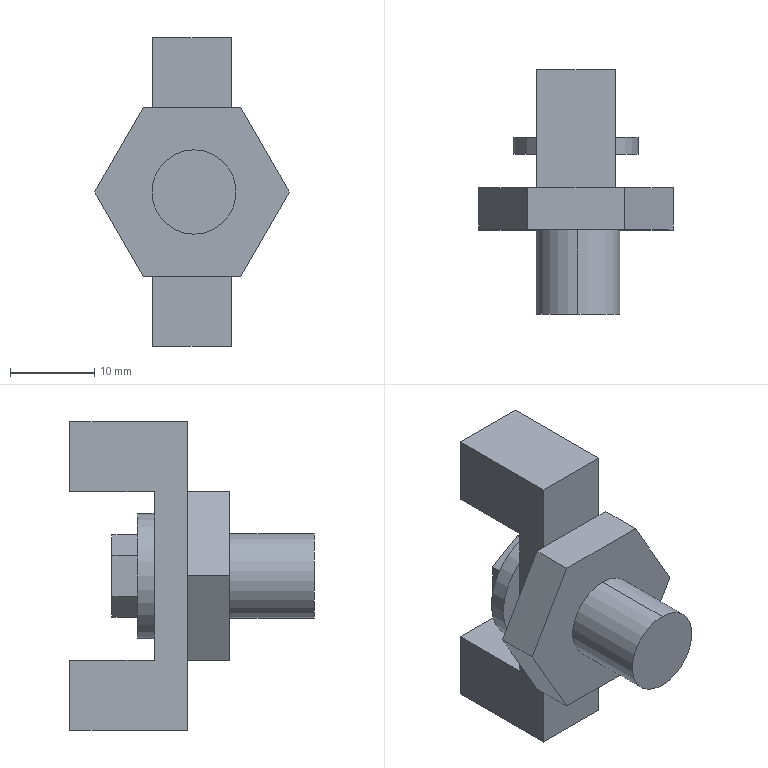Part | SolidWorks | features ICE 7, Extrusion 1 | 1 solid | 62 faces | box 23.094 x 29 x 36.628 mm | volume 5934 mm3 | plane 54 | cylinder 8 | commonest cylinder face diameters 5.701 x4 10 x2 14.848 x2